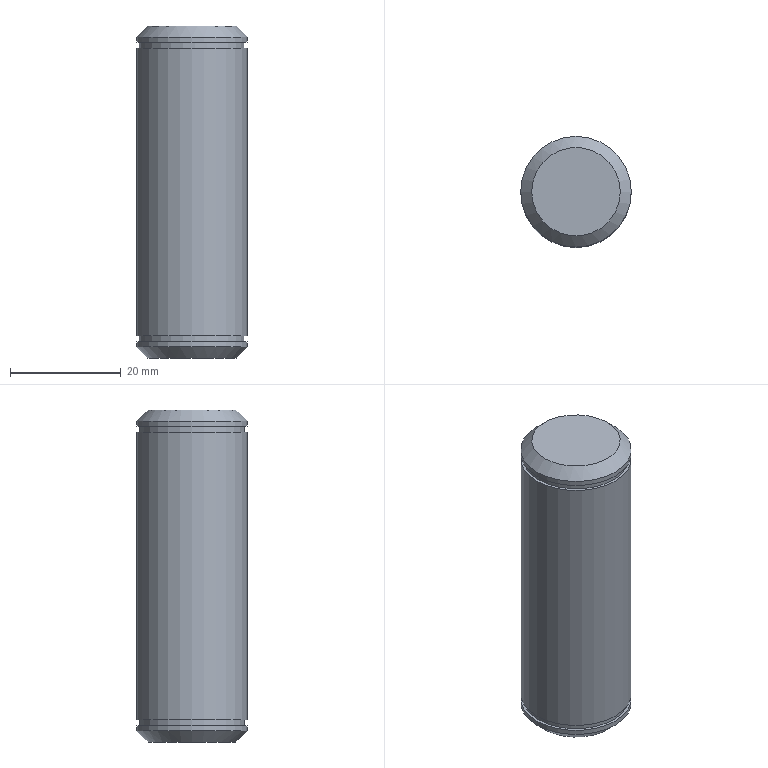Part | NX | features DATUM_CSYS 2, CHAMFER 1, SKETCH 1, SWP104 1 | 1 solid | 13 faces | box 20 x 20 x 60 mm | volume 18548 mm3 | plane 6 | cylinder 5 | cone 2 | commonest cylinder face diameters 20 x3 19 x2
STEP:
#1=CARTESIAN_POINT('',(-8.,0.,0.));
#2=VERTEX_POINT('',#1);
#3=CARTESIAN_POINT('',(0.,0.,0.));
#4=DIRECTION('',(0.,0.,-1.));
#5=DIRECTION('',(-1.,0.,0.));
#6=AXIS2_PLACEMENT_3D('',#3,#4,#5);
#7=CIRCLE('',#6,8.);
#8=EDGE_CURVE('',#2,#2,#7,.T.);
#9=ORIENTED_EDGE('',*,*,#8,.T.);
#10=EDGE_LOOP('',(#9));
#11=FACE_BOUND('',#10,.T.);
#12=CARTESIAN_POINT('',(0.,0.,0.));
#13=DIRECTION('',(0.,0.,-1.));
#14=DIRECTION('',(-1.,0.,0.));
#15=AXIS2_PLACEMENT_3D('',#12,#13,#14);
#16=PLANE('',#15);
#17=ADVANCED_FACE('',(#11),#16,.T.);
#18=CARTESIAN_POINT('',(-10.,0.,2.));
#19=VERTEX_POINT('',#18);
#20=CARTESIAN_POINT('',(0.,0.,2.));
#21=DIRECTION('',(0.,0.,-1.));
#22=DIRECTION('',(-1.,0.,0.));
#23=AXIS2_PLACEMENT_3D('',#20,#21,#22);
#24=CIRCLE('',#23,10.);
#25=EDGE_CURVE('',#19,#19,#24,.F.);
#26=ORIENTED_EDGE('',*,*,#25,.T.);
#27=EDGE_LOOP('',(#26));
#28=FACE_BOUND('',#27,.T.);
#29=CARTESIAN_POINT('',(-10.,0.,2.9));
#30=VERTEX_POINT('',#29);
#31=CARTESIAN_POINT('',(0.,0.,2.9));
#32=DIRECTION('',(0.,0.,-1.));
#33=DIRECTION('',(-1.,0.,0.));
#34=AXIS2_PLACEMENT_3D('',#31,#32,#33);
#35=CIRCLE('',#34,10.);
#36=EDGE_CURVE('',#30,#30,#35,.T.);
#37=ORIENTED_EDGE('',*,*,#36,.T.);
#38=EDGE_LOOP('',(#37));
#39=FACE_BOUND('',#38,.T.);
#40=CARTESIAN_POINT('',(0.,0.,0.));
#41=DIRECTION('',(0.,0.,-1.));
#42=DIRECTION('',(-1.,0.,0.));
#43=AXIS2_PLACEMENT_3D('',#40,#41,#42);
#44=CYLINDRICAL_SURFACE('',#43,10.);
#45=ADVANCED_FACE('',(#28,#39),#44,.T.);
#46=CARTESIAN_POINT('',(-9.5,0.,2.9));
#47=VERTEX_POINT('',#46);
#48=CARTESIAN_POINT('',(0.,0.,2.9));
#49=DIRECTION('',(0.,0.,-1.));
#50=DIRECTION('',(-1.,0.,0.));
#51=AXIS2_PLACEMENT_3D('',#48,#49,#50);
#52=CIRCLE('',#51,9.5);
#53=EDGE_CURVE('',#47,#47,#52,.T.);
#54=ORIENTED_EDGE('',*,*,#53,.T.);
#55=EDGE_LOOP('',(#54));
#56=FACE_BOUND('',#55,.T.);
#57=ORIENTED_EDGE('',*,*,#36,.F.);
#58=EDGE_LOOP('',(#57));
#59=FACE_BOUND('',#58,.T.);
#60=CARTESIAN_POINT('',(0.,10.,2.9));
#61=DIRECTION('',(0.,0.,1.));
#62=DIRECTION('',(1.,0.,0.));
#63=AXIS2_PLACEMENT_3D('',#60,#61,#62);
#64=PLANE('',#63);
#65=ADVANCED_FACE('',(#56,#59),#64,.T.);
#66=CARTESIAN_POINT('',(-9.5,0.,4.));
#67=VERTEX_POINT('',#66);
#68=CARTESIAN_POINT('',(0.,0.,4.));
#69=DIRECTION('',(0.,0.,-1.));
#70=DIRECTION('',(-1.,0.,0.));
#71=AXIS2_PLACEMENT_3D('',#68,#69,#70);
#72=CIRCLE('',#71,9.5);
#73=EDGE_CURVE('',#67,#67,#72,.T.);
#74=ORIENTED_EDGE('',*,*,#73,.T.);
#75=EDGE_LOOP('',(#74));
#76=FACE_BOUND('',#75,.T.);
#77=ORIENTED_EDGE('',*,*,#53,.F.);
#78=EDGE_LOOP('',(#77));
#79=FACE_BOUND('',#78,.T.);
#80=CARTESIAN_POINT('',(0.,0.,0.));
#81=DIRECTION('',(0.,0.,-1.));
#82=DIRECTION('',(-1.,0.,0.));
#83=AXIS2_PLACEMENT_3D('',#80,#81,#82);
#84=CYLINDRICAL_SURFACE('',#83,9.5);
#85=ADVANCED_FACE('',(#76,#79),#84,.T.);
#86=CARTESIAN_POINT('',(-10.,0.,4.));
#87=VERTEX_POINT('',#86);
#88=CARTESIAN_POINT('',(0.,0.,4.));
#89=DIRECTION('',(0.,0.,-1.));
#90=DIRECTION('',(-1.,0.,0.));
#91=AXIS2_PLACEMENT_3D('',#88,#89,#90);
#92=CIRCLE('',#91,10.);
#93=EDGE_CURVE('',#87,#87,#92,.T.);
#94=ORIENTED_EDGE('',*,*,#93,.T.);
#95=EDGE_LOOP('',(#94));
#96=FACE_BOUND('',#95,.T.);
#97=ORIENTED_EDGE('',*,*,#73,.F.);
#98=EDGE_LOOP('',(#97));
#99=FACE_BOUND('',#98,.T.);
#100=CARTESIAN_POINT('',(0.,9.5,4.));
#101=DIRECTION('',(0.,0.,-1.));
#102=DIRECTION('',(-1.,0.,0.));
#103=AXIS2_PLACEMENT_3D('',#100,#101,#102);
#104=PLANE('',#103);
#105=ADVANCED_FACE('',(#96,#99),#104,.T.);
#106=CARTESIAN_POINT('',(-10.,0.,56.));
#107=VERTEX_POINT('',#106);
#108=CARTESIAN_POINT('',(0.,0.,56.));
#109=DIRECTION('',(0.,0.,-1.));
#110=DIRECTION('',(-1.,0.,0.));
#111=AXIS2_PLACEMENT_3D('',#108,#109,#110);
#112=CIRCLE('',#111,10.);
#113=EDGE_CURVE('',#107,#107,#112,.T.);
#114=ORIENTED_EDGE('',*,*,#113,.T.);
#115=EDGE_LOOP('',(#114));
#116=FACE_BOUND('',#115,.T.);
#117=ORIENTED_EDGE('',*,*,#93,.F.);
#118=EDGE_LOOP('',(#117));
#119=FACE_BOUND('',#118,.T.);
#120=CARTESIAN_POINT('',(0.,0.,0.));
#121=DIRECTION('',(0.,0.,-1.));
#122=DIRECTION('',(-1.,0.,0.));
#123=AXIS2_PLACEMENT_3D('',#120,#121,#122);
#124=CYLINDRICAL_SURFACE('',#123,10.);
#125=ADVANCED_FACE('',(#116,#119),#124,.T.);
#126=CARTESIAN_POINT('',(-9.5,0.,56.));
#127=VERTEX_POINT('',#126);
#128=CARTESIAN_POINT('',(0.,0.,56.));
#129=DIRECTION('',(0.,0.,-1.));
#130=DIRECTION('',(-1.,0.,0.));
#131=AXIS2_PLACEMENT_3D('',#128,#129,#130);
#132=CIRCLE('',#131,9.5);
#133=EDGE_CURVE('',#127,#127,#132,.T.);
#134=ORIENTED_EDGE('',*,*,#133,.T.);
#135=EDGE_LOOP('',(#134));
#136=FACE_BOUND('',#135,.T.);
#137=ORIENTED_EDGE('',*,*,#113,.F.);
#138=EDGE_LOOP('',(#137));
#139=FACE_BOUND('',#138,.T.);
#140=CARTESIAN_POINT('',(0.,10.,56.));
#141=DIRECTION('',(0.,0.,1.));
#142=DIRECTION('',(1.,0.,0.));
#143=AXIS2_PLACEMENT_3D('',#140,#141,#142);
#144=PLANE('',#143);
#145=ADVANCED_FACE('',(#136,#139),#144,.T.);
#146=CARTESIAN_POINT('',(-9.5,0.,57.1));
#147=VERTEX_POINT('',#146);
#148=CARTESIAN_POINT('',(0.,0.,57.1));
#149=DIRECTION('',(0.,0.,-1.));
#150=DIRECTION('',(-1.,0.,0.));
#151=AXIS2_PLACEMENT_3D('',#148,#149,#150);
#152=CIRCLE('',#151,9.5);
#153=EDGE_CURVE('',#147,#147,#152,.T.);
#154=ORIENTED_EDGE('',*,*,#153,.T.);
#155=EDGE_LOOP('',(#154));
#156=FACE_BOUND('',#155,.T.);
#157=ORIENTED_EDGE('',*,*,#133,.F.);
#158=EDGE_LOOP('',(#157));
#159=FACE_BOUND('',#158,.T.);
#160=CARTESIAN_POINT('',(0.,0.,0.));
#161=DIRECTION('',(0.,0.,-1.));
#162=DIRECTION('',(-1.,0.,0.));
#163=AXIS2_PLACEMENT_3D('',#160,#161,#162);
#164=CYLINDRICAL_SURFACE('',#163,9.5);
#165=ADVANCED_FACE('',(#156,#159),#164,.T.);
#166=CARTESIAN_POINT('',(-10.,0.,57.1));
#167=VERTEX_POINT('',#166);
#168=CARTESIAN_POINT('',(0.,0.,57.1));
#169=DIRECTION('',(0.,0.,-1.));
#170=DIRECTION('',(-1.,0.,0.));
#171=AXIS2_PLACEMENT_3D('',#168,#169,#170);
#172=CIRCLE('',#171,10.);
#173=EDGE_CURVE('',#167,#167,#172,.T.);
#174=ORIENTED_EDGE('',*,*,#173,.T.);
#175=EDGE_LOOP('',(#174));
#176=FACE_BOUND('',#175,.T.);
#177=ORIENTED_EDGE('',*,*,#153,.F.);
#178=EDGE_LOOP('',(#177));
#179=FACE_BOUND('',#178,.T.);
#180=CARTESIAN_POINT('',(0.,9.5,57.1));
#181=DIRECTION('',(0.,0.,-1.));
#182=DIRECTION('',(-1.,0.,0.));
#183=AXIS2_PLACEMENT_3D('',#180,#181,#182);
#184=PLANE('',#183);
#185=ADVANCED_FACE('',(#176,#179),#184,.T.);
#186=CARTESIAN_POINT('',(10.,0.,58.));
#187=VERTEX_POINT('',#186);
#188=CARTESIAN_POINT('',(0.,0.,58.));
#189=DIRECTION('',(0.,0.,1.));
#190=DIRECTION('',(1.,0.,0.));
#191=AXIS2_PLACEMENT_3D('',#188,#189,#190);
#192=CIRCLE('',#191,10.);
#193=EDGE_CURVE('',#187,#187,#192,.F.);
#194=ORIENTED_EDGE('',*,*,#193,.T.);
#195=EDGE_LOOP('',(#194));
#196=FACE_BOUND('',#195,.T.);
#197=ORIENTED_EDGE('',*,*,#173,.F.);
#198=EDGE_LOOP('',(#197));
#199=FACE_BOUND('',#198,.T.);
#200=CARTESIAN_POINT('',(0.,0.,0.));
#201=DIRECTION('',(0.,0.,-1.));
#202=DIRECTION('',(-1.,0.,0.));
#203=AXIS2_PLACEMENT_3D('',#200,#201,#202);
#204=CYLINDRICAL_SURFACE('',#203,10.);
#205=ADVANCED_FACE('',(#196,#199),#204,.T.);
#206=CARTESIAN_POINT('',(8.,0.,60.));
#207=VERTEX_POINT('',#206);
#208=CARTESIAN_POINT('',(0.,0.,60.));
#209=DIRECTION('',(0.,0.,1.));
#210=DIRECTION('',(1.,0.,0.));
#211=AXIS2_PLACEMENT_3D('',#208,#209,#210);
#212=CIRCLE('',#211,8.);
#213=EDGE_CURVE('',#207,#207,#212,.T.);
#214=ORIENTED_EDGE('',*,*,#213,.T.);
#215=EDGE_LOOP('',(#214));
#216=FACE_BOUND('',#215,.T.);
#217=CARTESIAN_POINT('',(0.,10.,60.));
#218=DIRECTION('',(0.,0.,1.));
#219=DIRECTION('',(1.,0.,0.));
#220=AXIS2_PLACEMENT_3D('',#217,#218,#219);
#221=PLANE('',#220);
#222=ADVANCED_FACE('',(#216),#221,.T.);
#223=ORIENTED_EDGE('',*,*,#25,.F.);
#224=EDGE_LOOP('',(#223));
#225=FACE_BOUND('',#224,.T.);
#226=ORIENTED_EDGE('',*,*,#8,.F.);
#227=EDGE_LOOP('',(#226));
#228=FACE_BOUND('',#227,.T.);
#229=CARTESIAN_POINT('',(0.,0.,0.));
#230=DIRECTION('',(0.,0.,1.));
#231=DIRECTION('',(1.,0.,0.));
#232=AXIS2_PLACEMENT_3D('',#229,#230,#231);
#233=CONICAL_SURFACE('',#232,8.,0.7854);
#234=ADVANCED_FACE('',(#225,#228),#233,.T.);
#235=ORIENTED_EDGE('',*,*,#213,.F.);
#236=EDGE_LOOP('',(#235));
#237=FACE_BOUND('',#236,.T.);
#238=ORIENTED_EDGE('',*,*,#193,.F.);
#239=EDGE_LOOP('',(#238));
#240=FACE_BOUND('',#239,.T.);
#241=CARTESIAN_POINT('',(0.,0.,58.));
#242=DIRECTION('',(0.,0.,-1.));
#243=DIRECTION('',(-1.,0.,0.));
#244=AXIS2_PLACEMENT_3D('',#241,#242,#243);
#245=CONICAL_SURFACE('',#244,10.,0.7854);
#246=ADVANCED_FACE('',(#237,#240),#245,.T.);
#247=CLOSED_SHELL('',(#17,#45,#65,#85,#105,#125,#145,#165,#185,#205,#222,#234,#246));
#248=MANIFOLD_SOLID_BREP('',#247);
#249=(LENGTH_UNIT()NAMED_UNIT(*)SI_UNIT(.MILLI.,.METRE.));
#250=UNCERTAINTY_MEASURE_WITH_UNIT(LENGTH_MEASURE(0.00001),#249,'','');
#251=(NAMED_UNIT(*)PLANE_ANGLE_UNIT()SI_UNIT($,.RADIAN.));
#252=(NAMED_UNIT(*)SI_UNIT($,.STERADIAN.)SOLID_ANGLE_UNIT());
#253=(GEOMETRIC_REPRESENTATION_CONTEXT(3)GLOBAL_UNCERTAINTY_ASSIGNED_CONTEXT((#250))GLOBAL_UNIT_ASSIGNED_CONTEXT((#249,#251,#252))REPRESENTATION_CONTEXT('',''));
#254=ADVANCED_BREP_SHAPE_REPRESENTATION('',(#248),#253);